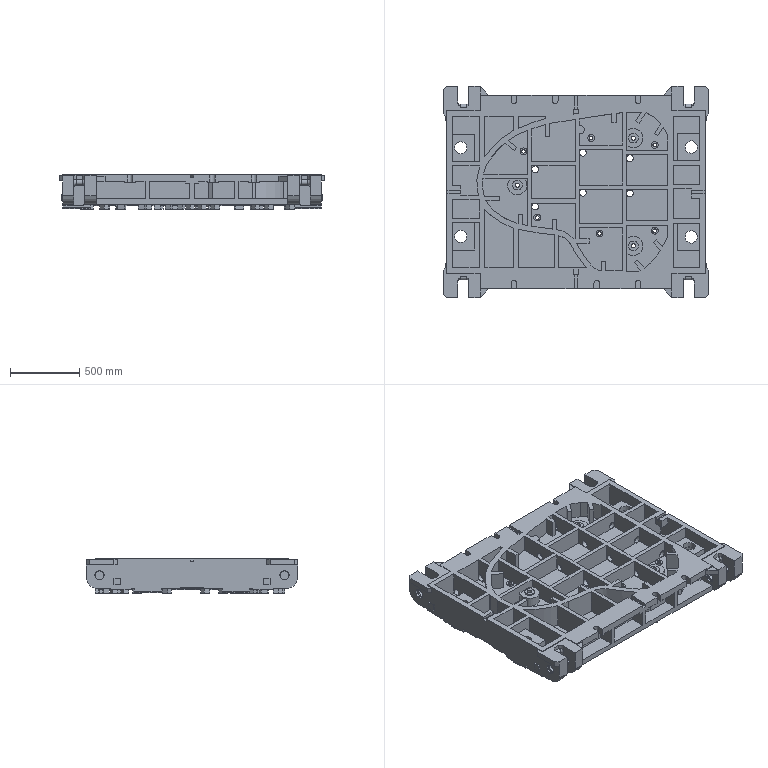Part | NX | features solid 2 | 1 solid | 1179 faces | box 1920 x 1530 x 250 mm | volume 261248586 mm3 | plane 914 | cylinder 203 | spline 54 | torus 8 | commonest cylinder face diameters 68 x48 50 x37 30 x18 64 x16 60 x15 20 x14